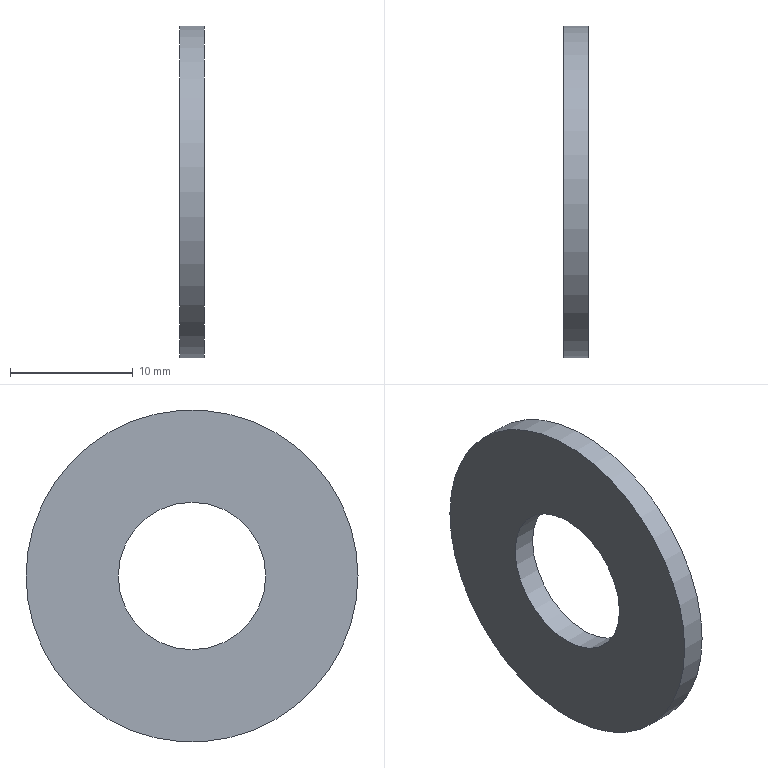Part | NX | features DATUM_CSYS 2, DATUM_PLANE 1, EXTRUDE 1, SKETCH 1 | 1 solid | 4 faces | box 2 x 27 x 27 mm | volume 918.916 mm3 | cylinder 2 | plane 2 | commonest cylinder face diameters 12 x1 27 x1
STEP:
#1=CARTESIAN_POINT('',(2.,13.5,0.));
#2=VERTEX_POINT('',#1);
#3=CARTESIAN_POINT('',(2.,0.,0.));
#4=DIRECTION('',(-1.,0.,0.));
#5=DIRECTION('',(0.,1.,0.));
#6=AXIS2_PLACEMENT_3D('',#3,#4,#5);
#7=CIRCLE('',#6,13.5);
#8=EDGE_CURVE('',#2,#2,#7,.T.);
#9=ORIENTED_EDGE('',*,*,#8,.T.);
#10=EDGE_LOOP('',(#9));
#11=FACE_BOUND('',#10,.T.);
#12=CARTESIAN_POINT('',(0.,13.5,0.));
#13=VERTEX_POINT('',#12);
#14=CARTESIAN_POINT('',(0.,0.,0.));
#15=DIRECTION('',(-1.,0.,0.));
#16=DIRECTION('',(0.,1.,0.));
#17=AXIS2_PLACEMENT_3D('',#14,#15,#16);
#18=CIRCLE('',#17,13.5);
#19=EDGE_CURVE('',#13,#13,#18,.T.);
#20=ORIENTED_EDGE('',*,*,#19,.F.);
#21=EDGE_LOOP('',(#20));
#22=FACE_BOUND('',#21,.T.);
#23=CARTESIAN_POINT('',(2.,0.,0.));
#24=DIRECTION('',(-1.,0.,0.));
#25=DIRECTION('',(0.,0.,1.));
#26=AXIS2_PLACEMENT_3D('',#23,#24,#25);
#27=CYLINDRICAL_SURFACE('',#26,13.5);
#28=ADVANCED_FACE('',(#11,#22),#27,.T.);
#29=CARTESIAN_POINT('',(2.,6.,0.));
#30=VERTEX_POINT('',#29);
#31=CARTESIAN_POINT('',(2.,0.,0.));
#32=DIRECTION('',(-1.,0.,0.));
#33=DIRECTION('',(0.,1.,0.));
#34=AXIS2_PLACEMENT_3D('',#31,#32,#33);
#35=CIRCLE('',#34,6.);
#36=EDGE_CURVE('',#30,#30,#35,.T.);
#37=ORIENTED_EDGE('',*,*,#36,.F.);
#38=EDGE_LOOP('',(#37));
#39=FACE_BOUND('',#38,.T.);
#40=CARTESIAN_POINT('',(0.,6.,0.));
#41=VERTEX_POINT('',#40);
#42=CARTESIAN_POINT('',(0.,0.,0.));
#43=DIRECTION('',(-1.,0.,0.));
#44=DIRECTION('',(0.,1.,0.));
#45=AXIS2_PLACEMENT_3D('',#42,#43,#44);
#46=CIRCLE('',#45,6.);
#47=EDGE_CURVE('',#41,#41,#46,.T.);
#48=ORIENTED_EDGE('',*,*,#47,.T.);
#49=EDGE_LOOP('',(#48));
#50=FACE_BOUND('',#49,.T.);
#51=CARTESIAN_POINT('',(2.,0.,0.));
#52=DIRECTION('',(-1.,0.,0.));
#53=DIRECTION('',(0.,0.,1.));
#54=AXIS2_PLACEMENT_3D('',#51,#52,#53);
#55=CYLINDRICAL_SURFACE('',#54,6.);
#56=ADVANCED_FACE('',(#39,#50),#55,.F.);
#57=ORIENTED_EDGE('',*,*,#8,.F.);
#58=EDGE_LOOP('',(#57));
#59=FACE_BOUND('',#58,.T.);
#60=ORIENTED_EDGE('',*,*,#36,.T.);
#61=EDGE_LOOP('',(#60));
#62=FACE_BOUND('',#61,.T.);
#63=CARTESIAN_POINT('',(2.,0.,0.));
#64=DIRECTION('',(-1.,0.,0.));
#65=DIRECTION('',(0.,0.,1.));
#66=AXIS2_PLACEMENT_3D('',#63,#64,#65);
#67=PLANE('',#66);
#68=ADVANCED_FACE('',(#59,#62),#67,.F.);
#69=ORIENTED_EDGE('',*,*,#19,.T.);
#70=EDGE_LOOP('',(#69));
#71=FACE_BOUND('',#70,.T.);
#72=ORIENTED_EDGE('',*,*,#47,.F.);
#73=EDGE_LOOP('',(#72));
#74=FACE_BOUND('',#73,.T.);
#75=CARTESIAN_POINT('',(0.,0.,0.));
#76=DIRECTION('',(-1.,0.,0.));
#77=DIRECTION('',(0.,0.,1.));
#78=AXIS2_PLACEMENT_3D('',#75,#76,#77);
#79=PLANE('',#78);
#80=ADVANCED_FACE('',(#71,#74),#79,.T.);
#81=CLOSED_SHELL('',(#28,#56,#68,#80));
#82=MANIFOLD_SOLID_BREP('',#81);
#83=(LENGTH_UNIT()NAMED_UNIT(*)SI_UNIT(.MILLI.,.METRE.));
#84=UNCERTAINTY_MEASURE_WITH_UNIT(LENGTH_MEASURE(0.00001),#83,'','');
#85=(NAMED_UNIT(*)PLANE_ANGLE_UNIT()SI_UNIT($,.RADIAN.));
#86=(NAMED_UNIT(*)SI_UNIT($,.STERADIAN.)SOLID_ANGLE_UNIT());
#87=(GEOMETRIC_REPRESENTATION_CONTEXT(3)GLOBAL_UNCERTAINTY_ASSIGNED_CONTEXT((#84))GLOBAL_UNIT_ASSIGNED_CONTEXT((#83,#85,#86))REPRESENTATION_CONTEXT('',''));
#88=ADVANCED_BREP_SHAPE_REPRESENTATION('',(#82),#87);